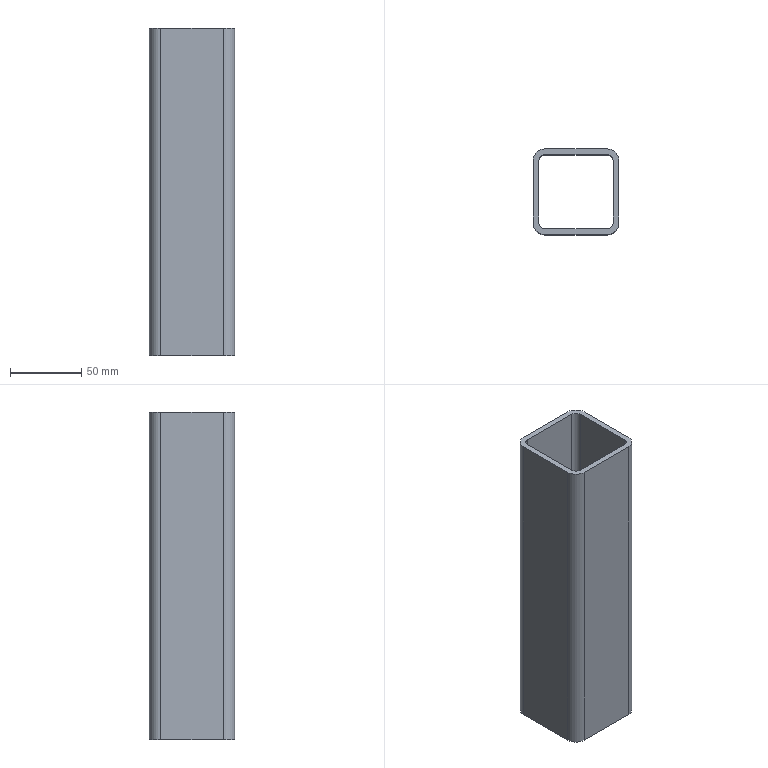Part | SolidWorks | features ICE 1, LibraryFeature 1 | 1 solid | 18 faces | box 60 x 60 x 230 mm | volume 196603 mm3 | plane 10 | cylinder 8 | commonest cylinder face diameters 8 x4 16 x4
STEP:
#1=CARTESIAN_POINT('',(22.,30.,0.));
#2=VERTEX_POINT('',#1);
#3=CARTESIAN_POINT('',(-22.,30.,0.));
#4=VERTEX_POINT('',#3);
#5=CARTESIAN_POINT('',(0.,30.,0.));
#6=DIRECTION('',(-1.,0.,0.));
#7=VECTOR('',#6,1000.);
#8=LINE('',#5,#7);
#9=EDGE_CURVE('',#2,#4,#8,.T.);
#10=ORIENTED_EDGE('',*,*,#9,.T.);
#11=CARTESIAN_POINT('',(-22.,30.,230.));
#12=VERTEX_POINT('',#11);
#13=CARTESIAN_POINT('',(-22.,30.,230.));
#14=DIRECTION('',(0.,0.,-1.));
#15=VECTOR('',#14,1000.);
#16=LINE('',#13,#15);
#17=EDGE_CURVE('',#12,#4,#16,.T.);
#18=ORIENTED_EDGE('',*,*,#17,.F.);
#19=CARTESIAN_POINT('',(22.,30.,230.));
#20=VERTEX_POINT('',#19);
#21=CARTESIAN_POINT('',(0.,30.,230.));
#22=DIRECTION('',(-1.,0.,0.));
#23=VECTOR('',#22,1000.);
#24=LINE('',#21,#23);
#25=EDGE_CURVE('',#20,#12,#24,.T.);
#26=ORIENTED_EDGE('',*,*,#25,.F.);
#27=CARTESIAN_POINT('',(22.,30.,230.));
#28=DIRECTION('',(0.,0.,-1.));
#29=VECTOR('',#28,1000.);
#30=LINE('',#27,#29);
#31=EDGE_CURVE('',#20,#2,#30,.T.);
#32=ORIENTED_EDGE('',*,*,#31,.T.);
#33=EDGE_LOOP('',(#10,#18,#26,#32));
#34=FACE_OUTER_BOUND('',#33,.T.);
#35=CARTESIAN_POINT('',(0.,30.,230.));
#36=DIRECTION('',(0.,-1.,0.));
#37=DIRECTION('',(0.,0.,-1.));
#38=AXIS2_PLACEMENT_3D('',#35,#36,#37);
#39=PLANE('',#38);
#40=ADVANCED_FACE('',(#34),#39,.F.);
#41=CARTESIAN_POINT('',(-30.,22.,0.));
#42=VERTEX_POINT('',#41);
#43=CARTESIAN_POINT('',(-22.,22.,0.));
#44=DIRECTION('',(0.,0.,1.));
#45=DIRECTION('',(1.,0.,0.));
#46=AXIS2_PLACEMENT_3D('',#43,#44,#45);
#47=CIRCLE('',#46,8.);
#48=EDGE_CURVE('',#4,#42,#47,.T.);
#49=ORIENTED_EDGE('',*,*,#48,.T.);
#50=CARTESIAN_POINT('',(-30.,22.,230.));
#51=VERTEX_POINT('',#50);
#52=CARTESIAN_POINT('',(-30.,22.,230.));
#53=DIRECTION('',(0.,0.,-1.));
#54=VECTOR('',#53,1000.);
#55=LINE('',#52,#54);
#56=EDGE_CURVE('',#51,#42,#55,.T.);
#57=ORIENTED_EDGE('',*,*,#56,.F.);
#58=CARTESIAN_POINT('',(-22.,22.,230.));
#59=DIRECTION('',(0.,0.,1.));
#60=DIRECTION('',(1.,0.,0.));
#61=AXIS2_PLACEMENT_3D('',#58,#59,#60);
#62=CIRCLE('',#61,8.);
#63=EDGE_CURVE('',#12,#51,#62,.T.);
#64=ORIENTED_EDGE('',*,*,#63,.F.);
#65=ORIENTED_EDGE('',*,*,#17,.T.);
#66=EDGE_LOOP('',(#49,#57,#64,#65));
#67=FACE_OUTER_BOUND('',#66,.T.);
#68=CARTESIAN_POINT('',(-22.,22.,230.));
#69=DIRECTION('',(0.,0.,-1.));
#70=DIRECTION('',(-1.,0.,0.));
#71=AXIS2_PLACEMENT_3D('',#68,#69,#70);
#72=CYLINDRICAL_SURFACE('',#71,8.);
#73=ADVANCED_FACE('',(#67),#72,.T.);
#74=CARTESIAN_POINT('',(-30.,-22.,0.));
#75=VERTEX_POINT('',#74);
#76=CARTESIAN_POINT('',(-30.,0.,0.));
#77=DIRECTION('',(0.,1.,0.));
#78=VECTOR('',#77,1000.);
#79=LINE('',#76,#78);
#80=EDGE_CURVE('',#75,#42,#79,.T.);
#81=ORIENTED_EDGE('',*,*,#80,.F.);
#82=CARTESIAN_POINT('',(-30.,-22.,230.));
#83=VERTEX_POINT('',#82);
#84=CARTESIAN_POINT('',(-30.,-22.,230.));
#85=DIRECTION('',(0.,0.,-1.));
#86=VECTOR('',#85,1000.);
#87=LINE('',#84,#86);
#88=EDGE_CURVE('',#83,#75,#87,.T.);
#89=ORIENTED_EDGE('',*,*,#88,.F.);
#90=CARTESIAN_POINT('',(-30.,0.,230.));
#91=DIRECTION('',(0.,1.,0.));
#92=VECTOR('',#91,1000.);
#93=LINE('',#90,#92);
#94=EDGE_CURVE('',#83,#51,#93,.T.);
#95=ORIENTED_EDGE('',*,*,#94,.T.);
#96=ORIENTED_EDGE('',*,*,#56,.T.);
#97=EDGE_LOOP('',(#81,#89,#95,#96));
#98=FACE_OUTER_BOUND('',#97,.T.);
#99=CARTESIAN_POINT('',(-30.,0.,230.));
#100=DIRECTION('',(-1.,0.,0.));
#101=DIRECTION('',(0.,0.,1.));
#102=AXIS2_PLACEMENT_3D('',#99,#100,#101);
#103=PLANE('',#102);
#104=ADVANCED_FACE('',(#98),#103,.T.);
#105=CARTESIAN_POINT('',(-22.,-30.,0.));
#106=VERTEX_POINT('',#105);
#107=CARTESIAN_POINT('',(-22.,-22.,0.));
#108=DIRECTION('',(0.,0.,1.));
#109=DIRECTION('',(1.,0.,0.));
#110=AXIS2_PLACEMENT_3D('',#107,#108,#109);
#111=CIRCLE('',#110,8.);
#112=EDGE_CURVE('',#75,#106,#111,.T.);
#113=ORIENTED_EDGE('',*,*,#112,.T.);
#114=CARTESIAN_POINT('',(-22.,-30.,230.));
#115=VERTEX_POINT('',#114);
#116=CARTESIAN_POINT('',(-22.,-30.,230.));
#117=DIRECTION('',(0.,0.,-1.));
#118=VECTOR('',#117,1000.);
#119=LINE('',#116,#118);
#120=EDGE_CURVE('',#115,#106,#119,.T.);
#121=ORIENTED_EDGE('',*,*,#120,.F.);
#122=CARTESIAN_POINT('',(-22.,-22.,230.));
#123=DIRECTION('',(0.,0.,1.));
#124=DIRECTION('',(1.,0.,0.));
#125=AXIS2_PLACEMENT_3D('',#122,#123,#124);
#126=CIRCLE('',#125,8.);
#127=EDGE_CURVE('',#83,#115,#126,.T.);
#128=ORIENTED_EDGE('',*,*,#127,.F.);
#129=ORIENTED_EDGE('',*,*,#88,.T.);
#130=EDGE_LOOP('',(#113,#121,#128,#129));
#131=FACE_OUTER_BOUND('',#130,.T.);
#132=CARTESIAN_POINT('',(-22.,-22.,230.));
#133=DIRECTION('',(0.,0.,-1.));
#134=DIRECTION('',(-1.,0.,0.));
#135=AXIS2_PLACEMENT_3D('',#132,#133,#134);
#136=CYLINDRICAL_SURFACE('',#135,8.);
#137=ADVANCED_FACE('',(#131),#136,.T.);
#138=CARTESIAN_POINT('',(22.,-30.,0.));
#139=VERTEX_POINT('',#138);
#140=CARTESIAN_POINT('',(0.,-30.,0.));
#141=DIRECTION('',(1.,0.,0.));
#142=VECTOR('',#141,1000.);
#143=LINE('',#140,#142);
#144=EDGE_CURVE('',#106,#139,#143,.T.);
#145=ORIENTED_EDGE('',*,*,#144,.T.);
#146=CARTESIAN_POINT('',(22.,-30.,230.));
#147=VERTEX_POINT('',#146);
#148=CARTESIAN_POINT('',(22.,-30.,230.));
#149=DIRECTION('',(0.,0.,-1.));
#150=VECTOR('',#149,1000.);
#151=LINE('',#148,#150);
#152=EDGE_CURVE('',#147,#139,#151,.T.);
#153=ORIENTED_EDGE('',*,*,#152,.F.);
#154=CARTESIAN_POINT('',(0.,-30.,230.));
#155=DIRECTION('',(1.,0.,0.));
#156=VECTOR('',#155,1000.);
#157=LINE('',#154,#156);
#158=EDGE_CURVE('',#115,#147,#157,.T.);
#159=ORIENTED_EDGE('',*,*,#158,.F.);
#160=ORIENTED_EDGE('',*,*,#120,.T.);
#161=EDGE_LOOP('',(#145,#153,#159,#160));
#162=FACE_OUTER_BOUND('',#161,.T.);
#163=CARTESIAN_POINT('',(0.,-30.,230.));
#164=DIRECTION('',(0.,1.,0.));
#165=DIRECTION('',(0.,0.,1.));
#166=AXIS2_PLACEMENT_3D('',#163,#164,#165);
#167=PLANE('',#166);
#168=ADVANCED_FACE('',(#162),#167,.F.);
#169=CARTESIAN_POINT('',(30.,-22.,0.));
#170=VERTEX_POINT('',#169);
#171=CARTESIAN_POINT('',(22.,-22.,0.));
#172=DIRECTION('',(0.,0.,1.));
#173=DIRECTION('',(1.,0.,0.));
#174=AXIS2_PLACEMENT_3D('',#171,#172,#173);
#175=CIRCLE('',#174,8.);
#176=EDGE_CURVE('',#139,#170,#175,.T.);
#177=ORIENTED_EDGE('',*,*,#176,.T.);
#178=CARTESIAN_POINT('',(30.,-22.,230.));
#179=VERTEX_POINT('',#178);
#180=CARTESIAN_POINT('',(30.,-22.,230.));
#181=DIRECTION('',(0.,0.,-1.));
#182=VECTOR('',#181,1000.);
#183=LINE('',#180,#182);
#184=EDGE_CURVE('',#179,#170,#183,.T.);
#185=ORIENTED_EDGE('',*,*,#184,.F.);
#186=CARTESIAN_POINT('',(22.,-22.,230.));
#187=DIRECTION('',(0.,0.,1.));
#188=DIRECTION('',(1.,0.,0.));
#189=AXIS2_PLACEMENT_3D('',#186,#187,#188);
#190=CIRCLE('',#189,8.);
#191=EDGE_CURVE('',#147,#179,#190,.T.);
#192=ORIENTED_EDGE('',*,*,#191,.F.);
#193=ORIENTED_EDGE('',*,*,#152,.T.);
#194=EDGE_LOOP('',(#177,#185,#192,#193));
#195=FACE_OUTER_BOUND('',#194,.T.);
#196=CARTESIAN_POINT('',(22.,-22.,230.));
#197=DIRECTION('',(0.,0.,-1.));
#198=DIRECTION('',(-1.,0.,0.));
#199=AXIS2_PLACEMENT_3D('',#196,#197,#198);
#200=CYLINDRICAL_SURFACE('',#199,8.);
#201=ADVANCED_FACE('',(#195),#200,.T.);
#202=CARTESIAN_POINT('',(30.,22.,0.));
#203=VERTEX_POINT('',#202);
#204=CARTESIAN_POINT('',(30.,0.,0.));
#205=DIRECTION('',(0.,-1.,0.));
#206=VECTOR('',#205,1000.);
#207=LINE('',#204,#206);
#208=EDGE_CURVE('',#203,#170,#207,.T.);
#209=ORIENTED_EDGE('',*,*,#208,.F.);
#210=CARTESIAN_POINT('',(30.,22.,230.));
#211=VERTEX_POINT('',#210);
#212=CARTESIAN_POINT('',(30.,22.,230.));
#213=DIRECTION('',(0.,0.,-1.));
#214=VECTOR('',#213,1000.);
#215=LINE('',#212,#214);
#216=EDGE_CURVE('',#211,#203,#215,.T.);
#217=ORIENTED_EDGE('',*,*,#216,.F.);
#218=CARTESIAN_POINT('',(30.,0.,230.));
#219=DIRECTION('',(0.,-1.,0.));
#220=VECTOR('',#219,1000.);
#221=LINE('',#218,#220);
#222=EDGE_CURVE('',#211,#179,#221,.T.);
#223=ORIENTED_EDGE('',*,*,#222,.T.);
#224=ORIENTED_EDGE('',*,*,#184,.T.);
#225=EDGE_LOOP('',(#209,#217,#223,#224));
#226=FACE_OUTER_BOUND('',#225,.T.);
#227=CARTESIAN_POINT('',(30.,0.,230.));
#228=DIRECTION('',(1.,0.,0.));
#229=DIRECTION('',(0.,0.,-1.));
#230=AXIS2_PLACEMENT_3D('',#227,#228,#229);
#231=PLANE('',#230);
#232=ADVANCED_FACE('',(#226),#231,.T.);
#233=CARTESIAN_POINT('',(-26.,-22.,0.));
#234=VERTEX_POINT('',#233);
#235=CARTESIAN_POINT('',(-22.,-26.,0.));
#236=VERTEX_POINT('',#235);
#237=CARTESIAN_POINT('',(-22.,-22.,0.));
#238=DIRECTION('',(0.,0.,1.));
#239=DIRECTION('',(1.,0.,0.));
#240=AXIS2_PLACEMENT_3D('',#237,#238,#239);
#241=CIRCLE('',#240,4.);
#242=EDGE_CURVE('',#234,#236,#241,.T.);
#243=ORIENTED_EDGE('',*,*,#242,.F.);
#244=CARTESIAN_POINT('',(-26.,-22.,230.));
#245=VERTEX_POINT('',#244);
#246=CARTESIAN_POINT('',(-26.,-22.,230.));
#247=DIRECTION('',(0.,0.,-1.));
#248=VECTOR('',#247,1000.);
#249=LINE('',#246,#248);
#250=EDGE_CURVE('',#245,#234,#249,.T.);
#251=ORIENTED_EDGE('',*,*,#250,.F.);
#252=CARTESIAN_POINT('',(-22.,-26.,230.));
#253=VERTEX_POINT('',#252);
#254=CARTESIAN_POINT('',(-22.,-22.,230.));
#255=DIRECTION('',(0.,0.,1.));
#256=DIRECTION('',(1.,0.,0.));
#257=AXIS2_PLACEMENT_3D('',#254,#255,#256);
#258=CIRCLE('',#257,4.);
#259=EDGE_CURVE('',#245,#253,#258,.T.);
#260=ORIENTED_EDGE('',*,*,#259,.T.);
#261=CARTESIAN_POINT('',(-22.,-26.,230.));
#262=DIRECTION('',(0.,0.,-1.));
#263=VECTOR('',#262,1000.);
#264=LINE('',#261,#263);
#265=EDGE_CURVE('',#253,#236,#264,.T.);
#266=ORIENTED_EDGE('',*,*,#265,.T.);
#267=EDGE_LOOP('',(#243,#251,#260,#266));
#268=FACE_OUTER_BOUND('',#267,.T.);
#269=CARTESIAN_POINT('',(-22.,-22.,230.));
#270=DIRECTION('',(0.,0.,-1.));
#271=DIRECTION('',(-1.,0.,0.));
#272=AXIS2_PLACEMENT_3D('',#269,#270,#271);
#273=CYLINDRICAL_SURFACE('',#272,4.);
#274=ADVANCED_FACE('',(#268),#273,.F.);
#275=CARTESIAN_POINT('',(-26.,22.,0.));
#276=VERTEX_POINT('',#275);
#277=CARTESIAN_POINT('',(-26.,0.,0.));
#278=DIRECTION('',(0.,1.,0.));
#279=VECTOR('',#278,1000.);
#280=LINE('',#277,#279);
#281=EDGE_CURVE('',#234,#276,#280,.T.);
#282=ORIENTED_EDGE('',*,*,#281,.T.);
#283=CARTESIAN_POINT('',(-26.,22.,230.));
#284=VERTEX_POINT('',#283);
#285=CARTESIAN_POINT('',(-26.,22.,230.));
#286=DIRECTION('',(0.,0.,-1.));
#287=VECTOR('',#286,1000.);
#288=LINE('',#285,#287);
#289=EDGE_CURVE('',#284,#276,#288,.T.);
#290=ORIENTED_EDGE('',*,*,#289,.F.);
#291=CARTESIAN_POINT('',(-26.,0.,230.));
#292=DIRECTION('',(0.,1.,0.));
#293=VECTOR('',#292,1000.);
#294=LINE('',#291,#293);
#295=EDGE_CURVE('',#245,#284,#294,.T.);
#296=ORIENTED_EDGE('',*,*,#295,.F.);
#297=ORIENTED_EDGE('',*,*,#250,.T.);
#298=EDGE_LOOP('',(#282,#290,#296,#297));
#299=FACE_OUTER_BOUND('',#298,.T.);
#300=CARTESIAN_POINT('',(-26.,0.,230.));
#301=DIRECTION('',(-1.,0.,0.));
#302=DIRECTION('',(0.,0.,1.));
#303=AXIS2_PLACEMENT_3D('',#300,#301,#302);
#304=PLANE('',#303);
#305=ADVANCED_FACE('',(#299),#304,.F.);
#306=CARTESIAN_POINT('',(-22.,26.,0.));
#307=VERTEX_POINT('',#306);
#308=CARTESIAN_POINT('',(-22.,22.,0.));
#309=DIRECTION('',(0.,0.,1.));
#310=DIRECTION('',(1.,0.,0.));
#311=AXIS2_PLACEMENT_3D('',#308,#309,#310);
#312=CIRCLE('',#311,4.);
#313=EDGE_CURVE('',#307,#276,#312,.T.);
#314=ORIENTED_EDGE('',*,*,#313,.F.);
#315=CARTESIAN_POINT('',(-22.,26.,230.));
#316=VERTEX_POINT('',#315);
#317=CARTESIAN_POINT('',(-22.,26.,230.));
#318=DIRECTION('',(0.,0.,-1.));
#319=VECTOR('',#318,1000.);
#320=LINE('',#317,#319);
#321=EDGE_CURVE('',#316,#307,#320,.T.);
#322=ORIENTED_EDGE('',*,*,#321,.F.);
#323=CARTESIAN_POINT('',(-22.,22.,230.));
#324=DIRECTION('',(0.,0.,1.));
#325=DIRECTION('',(1.,0.,0.));
#326=AXIS2_PLACEMENT_3D('',#323,#324,#325);
#327=CIRCLE('',#326,4.);
#328=EDGE_CURVE('',#316,#284,#327,.T.);
#329=ORIENTED_EDGE('',*,*,#328,.T.);
#330=ORIENTED_EDGE('',*,*,#289,.T.);
#331=EDGE_LOOP('',(#314,#322,#329,#330));
#332=FACE_OUTER_BOUND('',#331,.T.);
#333=CARTESIAN_POINT('',(-22.,22.,230.));
#334=DIRECTION('',(0.,0.,-1.));
#335=DIRECTION('',(-1.,0.,0.));
#336=AXIS2_PLACEMENT_3D('',#333,#334,#335);
#337=CYLINDRICAL_SURFACE('',#336,4.);
#338=ADVANCED_FACE('',(#332),#337,.F.);
#339=CARTESIAN_POINT('',(22.,26.,0.));
#340=VERTEX_POINT('',#339);
#341=CARTESIAN_POINT('',(0.,26.,0.));
#342=DIRECTION('',(-1.,0.,0.));
#343=VECTOR('',#342,1000.);
#344=LINE('',#341,#343);
#345=EDGE_CURVE('',#340,#307,#344,.T.);
#346=ORIENTED_EDGE('',*,*,#345,.F.);
#347=CARTESIAN_POINT('',(22.,26.,230.));
#348=VERTEX_POINT('',#347);
#349=CARTESIAN_POINT('',(22.,26.,230.));
#350=DIRECTION('',(0.,0.,-1.));
#351=VECTOR('',#350,1000.);
#352=LINE('',#349,#351);
#353=EDGE_CURVE('',#348,#340,#352,.T.);
#354=ORIENTED_EDGE('',*,*,#353,.F.);
#355=CARTESIAN_POINT('',(0.,26.,230.));
#356=DIRECTION('',(-1.,0.,0.));
#357=VECTOR('',#356,1000.);
#358=LINE('',#355,#357);
#359=EDGE_CURVE('',#348,#316,#358,.T.);
#360=ORIENTED_EDGE('',*,*,#359,.T.);
#361=ORIENTED_EDGE('',*,*,#321,.T.);
#362=EDGE_LOOP('',(#346,#354,#360,#361));
#363=FACE_OUTER_BOUND('',#362,.T.);
#364=CARTESIAN_POINT('',(0.,26.,230.));
#365=DIRECTION('',(0.,-1.,0.));
#366=DIRECTION('',(0.,0.,-1.));
#367=AXIS2_PLACEMENT_3D('',#364,#365,#366);
#368=PLANE('',#367);
#369=ADVANCED_FACE('',(#363),#368,.T.);
#370=CARTESIAN_POINT('',(26.,22.,0.));
#371=VERTEX_POINT('',#370);
#372=CARTESIAN_POINT('',(22.,22.,0.));
#373=DIRECTION('',(0.,0.,1.));
#374=DIRECTION('',(1.,0.,0.));
#375=AXIS2_PLACEMENT_3D('',#372,#373,#374);
#376=CIRCLE('',#375,4.);
#377=EDGE_CURVE('',#371,#340,#376,.T.);
#378=ORIENTED_EDGE('',*,*,#377,.F.);
#379=CARTESIAN_POINT('',(26.,22.,230.));
#380=VERTEX_POINT('',#379);
#381=CARTESIAN_POINT('',(26.,22.,230.));
#382=DIRECTION('',(0.,0.,-1.));
#383=VECTOR('',#382,1000.);
#384=LINE('',#381,#383);
#385=EDGE_CURVE('',#380,#371,#384,.T.);
#386=ORIENTED_EDGE('',*,*,#385,.F.);
#387=CARTESIAN_POINT('',(22.,22.,230.));
#388=DIRECTION('',(0.,0.,1.));
#389=DIRECTION('',(1.,0.,0.));
#390=AXIS2_PLACEMENT_3D('',#387,#388,#389);
#391=CIRCLE('',#390,4.);
#392=EDGE_CURVE('',#380,#348,#391,.T.);
#393=ORIENTED_EDGE('',*,*,#392,.T.);
#394=ORIENTED_EDGE('',*,*,#353,.T.);
#395=EDGE_LOOP('',(#378,#386,#393,#394));
#396=FACE_OUTER_BOUND('',#395,.T.);
#397=CARTESIAN_POINT('',(22.,22.,230.));
#398=DIRECTION('',(0.,0.,-1.));
#399=DIRECTION('',(-1.,0.,0.));
#400=AXIS2_PLACEMENT_3D('',#397,#398,#399);
#401=CYLINDRICAL_SURFACE('',#400,4.);
#402=ADVANCED_FACE('',(#396),#401,.F.);
#403=CARTESIAN_POINT('',(26.,-22.,0.));
#404=VERTEX_POINT('',#403);
#405=CARTESIAN_POINT('',(26.,0.,0.));
#406=DIRECTION('',(0.,-1.,0.));
#407=VECTOR('',#406,1000.);
#408=LINE('',#405,#407);
#409=EDGE_CURVE('',#371,#404,#408,.T.);
#410=ORIENTED_EDGE('',*,*,#409,.T.);
#411=CARTESIAN_POINT('',(26.,-22.,230.));
#412=VERTEX_POINT('',#411);
#413=CARTESIAN_POINT('',(26.,-22.,230.));
#414=DIRECTION('',(0.,0.,-1.));
#415=VECTOR('',#414,1000.);
#416=LINE('',#413,#415);
#417=EDGE_CURVE('',#412,#404,#416,.T.);
#418=ORIENTED_EDGE('',*,*,#417,.F.);
#419=CARTESIAN_POINT('',(26.,0.,230.));
#420=DIRECTION('',(0.,-1.,0.));
#421=VECTOR('',#420,1000.);
#422=LINE('',#419,#421);
#423=EDGE_CURVE('',#380,#412,#422,.T.);
#424=ORIENTED_EDGE('',*,*,#423,.F.);
#425=ORIENTED_EDGE('',*,*,#385,.T.);
#426=EDGE_LOOP('',(#410,#418,#424,#425));
#427=FACE_OUTER_BOUND('',#426,.T.);
#428=CARTESIAN_POINT('',(26.,0.,230.));
#429=DIRECTION('',(1.,0.,0.));
#430=DIRECTION('',(0.,0.,-1.));
#431=AXIS2_PLACEMENT_3D('',#428,#429,#430);
#432=PLANE('',#431);
#433=ADVANCED_FACE('',(#427),#432,.F.);
#434=CARTESIAN_POINT('',(22.,-26.,0.));
#435=VERTEX_POINT('',#434);
#436=CARTESIAN_POINT('',(22.,-22.,0.));
#437=DIRECTION('',(0.,0.,1.));
#438=DIRECTION('',(1.,0.,0.));
#439=AXIS2_PLACEMENT_3D('',#436,#437,#438);
#440=CIRCLE('',#439,4.);
#441=EDGE_CURVE('',#435,#404,#440,.T.);
#442=ORIENTED_EDGE('',*,*,#441,.F.);
#443=CARTESIAN_POINT('',(22.,-26.,230.));
#444=VERTEX_POINT('',#443);
#445=CARTESIAN_POINT('',(22.,-26.,230.));
#446=DIRECTION('',(0.,0.,-1.));
#447=VECTOR('',#446,1000.);
#448=LINE('',#445,#447);
#449=EDGE_CURVE('',#444,#435,#448,.T.);
#450=ORIENTED_EDGE('',*,*,#449,.F.);
#451=CARTESIAN_POINT('',(22.,-22.,230.));
#452=DIRECTION('',(0.,0.,1.));
#453=DIRECTION('',(1.,0.,0.));
#454=AXIS2_PLACEMENT_3D('',#451,#452,#453);
#455=CIRCLE('',#454,4.);
#456=EDGE_CURVE('',#444,#412,#455,.T.);
#457=ORIENTED_EDGE('',*,*,#456,.T.);
#458=ORIENTED_EDGE('',*,*,#417,.T.);
#459=EDGE_LOOP('',(#442,#450,#457,#458));
#460=FACE_OUTER_BOUND('',#459,.T.);
#461=CARTESIAN_POINT('',(22.,-22.,230.));
#462=DIRECTION('',(0.,0.,-1.));
#463=DIRECTION('',(-1.,0.,0.));
#464=AXIS2_PLACEMENT_3D('',#461,#462,#463);
#465=CYLINDRICAL_SURFACE('',#464,4.);
#466=ADVANCED_FACE('',(#460),#465,.F.);
#467=CARTESIAN_POINT('',(0.,-26.,0.));
#468=DIRECTION('',(1.,0.,0.));
#469=VECTOR('',#468,1000.);
#470=LINE('',#467,#469);
#471=EDGE_CURVE('',#236,#435,#470,.T.);
#472=ORIENTED_EDGE('',*,*,#471,.F.);
#473=ORIENTED_EDGE('',*,*,#265,.F.);
#474=CARTESIAN_POINT('',(0.,-26.,230.));
#475=DIRECTION('',(1.,0.,0.));
#476=VECTOR('',#475,1000.);
#477=LINE('',#474,#476);
#478=EDGE_CURVE('',#253,#444,#477,.T.);
#479=ORIENTED_EDGE('',*,*,#478,.T.);
#480=ORIENTED_EDGE('',*,*,#449,.T.);
#481=EDGE_LOOP('',(#472,#473,#479,#480));
#482=FACE_OUTER_BOUND('',#481,.T.);
#483=CARTESIAN_POINT('',(0.,-26.,230.));
#484=DIRECTION('',(0.,1.,0.));
#485=DIRECTION('',(0.,0.,1.));
#486=AXIS2_PLACEMENT_3D('',#483,#484,#485);
#487=PLANE('',#486);
#488=ADVANCED_FACE('',(#482),#487,.T.);
#489=CARTESIAN_POINT('',(22.,22.,0.));
#490=DIRECTION('',(0.,0.,1.));
#491=DIRECTION('',(1.,0.,0.));
#492=AXIS2_PLACEMENT_3D('',#489,#490,#491);
#493=CIRCLE('',#492,8.);
#494=EDGE_CURVE('',#203,#2,#493,.T.);
#495=ORIENTED_EDGE('',*,*,#494,.T.);
#496=ORIENTED_EDGE('',*,*,#31,.F.);
#497=CARTESIAN_POINT('',(22.,22.,230.));
#498=DIRECTION('',(0.,0.,1.));
#499=DIRECTION('',(1.,0.,0.));
#500=AXIS2_PLACEMENT_3D('',#497,#498,#499);
#501=CIRCLE('',#500,8.);
#502=EDGE_CURVE('',#211,#20,#501,.T.);
#503=ORIENTED_EDGE('',*,*,#502,.F.);
#504=ORIENTED_EDGE('',*,*,#216,.T.);
#505=EDGE_LOOP('',(#495,#496,#503,#504));
#506=FACE_OUTER_BOUND('',#505,.T.);
#507=CARTESIAN_POINT('',(22.,22.,230.));
#508=DIRECTION('',(0.,0.,-1.));
#509=DIRECTION('',(-1.,0.,0.));
#510=AXIS2_PLACEMENT_3D('',#507,#508,#509);
#511=CYLINDRICAL_SURFACE('',#510,8.);
#512=ADVANCED_FACE('',(#506),#511,.T.);
#513=ORIENTED_EDGE('',*,*,#259,.F.);
#514=ORIENTED_EDGE('',*,*,#295,.T.);
#515=ORIENTED_EDGE('',*,*,#328,.F.);
#516=ORIENTED_EDGE('',*,*,#359,.F.);
#517=ORIENTED_EDGE('',*,*,#392,.F.);
#518=ORIENTED_EDGE('',*,*,#423,.T.);
#519=ORIENTED_EDGE('',*,*,#456,.F.);
#520=ORIENTED_EDGE('',*,*,#478,.F.);
#521=EDGE_LOOP('',(#513,#514,#515,#516,#517,#518,#519,#520));
#522=FACE_BOUND('',#521,.T.);
#523=ORIENTED_EDGE('',*,*,#25,.T.);
#524=ORIENTED_EDGE('',*,*,#63,.T.);
#525=ORIENTED_EDGE('',*,*,#94,.F.);
#526=ORIENTED_EDGE('',*,*,#127,.T.);
#527=ORIENTED_EDGE('',*,*,#158,.T.);
#528=ORIENTED_EDGE('',*,*,#191,.T.);
#529=ORIENTED_EDGE('',*,*,#222,.F.);
#530=ORIENTED_EDGE('',*,*,#502,.T.);
#531=EDGE_LOOP('',(#523,#524,#525,#526,#527,#528,#529,#530));
#532=FACE_OUTER_BOUND('',#531,.T.);
#533=CARTESIAN_POINT('',(0.,0.,230.));
#534=DIRECTION('',(0.,0.,1.));
#535=DIRECTION('',(1.,0.,0.));
#536=AXIS2_PLACEMENT_3D('',#533,#534,#535);
#537=PLANE('',#536);
#538=ADVANCED_FACE('',(#522,#532),#537,.T.);
#539=ORIENTED_EDGE('',*,*,#242,.T.);
#540=ORIENTED_EDGE('',*,*,#471,.T.);
#541=ORIENTED_EDGE('',*,*,#441,.T.);
#542=ORIENTED_EDGE('',*,*,#409,.F.);
#543=ORIENTED_EDGE('',*,*,#377,.T.);
#544=ORIENTED_EDGE('',*,*,#345,.T.);
#545=ORIENTED_EDGE('',*,*,#313,.T.);
#546=ORIENTED_EDGE('',*,*,#281,.F.);
#547=EDGE_LOOP('',(#539,#540,#541,#542,#543,#544,#545,#546));
#548=FACE_BOUND('',#547,.T.);
#549=ORIENTED_EDGE('',*,*,#9,.F.);
#550=ORIENTED_EDGE('',*,*,#494,.F.);
#551=ORIENTED_EDGE('',*,*,#208,.T.);
#552=ORIENTED_EDGE('',*,*,#176,.F.);
#553=ORIENTED_EDGE('',*,*,#144,.F.);
#554=ORIENTED_EDGE('',*,*,#112,.F.);
#555=ORIENTED_EDGE('',*,*,#80,.T.);
#556=ORIENTED_EDGE('',*,*,#48,.F.);
#557=EDGE_LOOP('',(#549,#550,#551,#552,#553,#554,#555,#556));
#558=FACE_OUTER_BOUND('',#557,.T.);
#559=CARTESIAN_POINT('',(0.,0.,0.));
#560=DIRECTION('',(0.,0.,1.));
#561=DIRECTION('',(1.,0.,0.));
#562=AXIS2_PLACEMENT_3D('',#559,#560,#561);
#563=PLANE('',#562);
#564=ADVANCED_FACE('',(#548,#558),#563,.F.);
#565=CLOSED_SHELL('',(#40,#73,#104,#137,#168,#201,#232,#274,#305,#338,#369,#402,#433,#466,#488,#512,#538,#564));
#566=MANIFOLD_SOLID_BREP('',#565);
#567=CARTESIAN_POINT('',(0.,0.,0.));
#568=DIRECTION('',(0.,0.,1.));
#569=DIRECTION('',(1.,0.,0.));
#570=AXIS2_PLACEMENT_3D('',#567,#568,#569);
#571=(LENGTH_UNIT()NAMED_UNIT(*)SI_UNIT(.MILLI.,.METRE.));
#572=UNCERTAINTY_MEASURE_WITH_UNIT(LENGTH_MEASURE(0.00001),#571,'','');
#573=(NAMED_UNIT(*)PLANE_ANGLE_UNIT()SI_UNIT($,.RADIAN.));
#574=(NAMED_UNIT(*)SI_UNIT($,.STERADIAN.)SOLID_ANGLE_UNIT());
#575=(GEOMETRIC_REPRESENTATION_CONTEXT(3)GLOBAL_UNCERTAINTY_ASSIGNED_CONTEXT((#572))GLOBAL_UNIT_ASSIGNED_CONTEXT((#571,#573,#574))REPRESENTATION_CONTEXT('',''));
#576=ADVANCED_BREP_SHAPE_REPRESENTATION('',(#566,#570),#575);